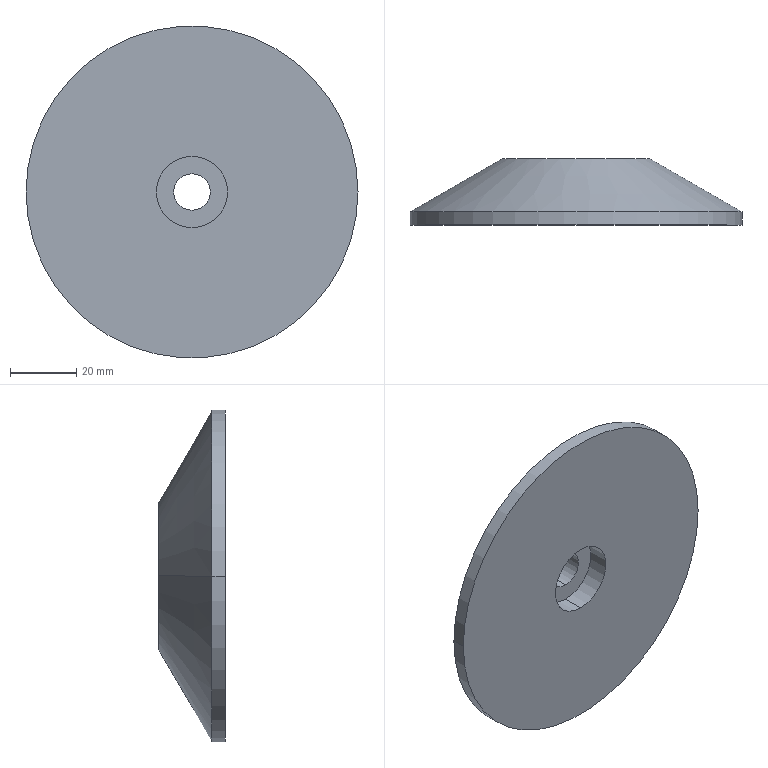Part | STEP file | Microwave Drying Flat Conveyor-CN2500x400-105-106 | 1 solid | 11 faces | box 100 x 20 x 100 mm | volume 96687 mm3 | cylinder 6 | plane 3 | cone 2 | commonest cylinder face diameters 11 x2 21.475 x2 100 x2
STEP:
#1=CARTESIAN_POINT('',(0.,6.4,10.738));
#2=VERTEX_POINT('',#1);
#3=CARTESIAN_POINT('',(0.,6.4,-10.738));
#4=VERTEX_POINT('',#3);
#5=CARTESIAN_POINT('',(0.,6.4,0.));
#6=DIRECTION('',(0.,-1.,0.));
#7=DIRECTION('',(0.,0.,-1.));
#8=AXIS2_PLACEMENT_3D('',#5,#6,#7);
#9=CIRCLE('',#8,10.738);
#10=EDGE_CURVE('',#2,#4,#9,.T.);
#11=ORIENTED_EDGE('',*,*,#10,.F.);
#12=CARTESIAN_POINT('',(0.,0.,10.737));
#13=VERTEX_POINT('',#12);
#14=CARTESIAN_POINT('',(0.,0.,10.738));
#15=DIRECTION('',(0.,-1.,0.));
#16=VECTOR('',#15,1000.);
#17=LINE('',#14,#16);
#18=EDGE_CURVE('',#2,#13,#17,.T.);
#19=ORIENTED_EDGE('',*,*,#18,.T.);
#20=CARTESIAN_POINT('',(0.,0.,-10.737));
#21=VERTEX_POINT('',#20);
#22=CARTESIAN_POINT('',(0.,0.,0.));
#23=DIRECTION('',(0.,-1.,0.));
#24=DIRECTION('',(0.,0.,-1.));
#25=AXIS2_PLACEMENT_3D('',#22,#23,#24);
#26=CIRCLE('',#25,10.737);
#27=EDGE_CURVE('',#13,#21,#26,.T.);
#28=ORIENTED_EDGE('',*,*,#27,.T.);
#29=CARTESIAN_POINT('',(0.,0.,-10.738));
#30=DIRECTION('',(0.,-1.,0.));
#31=VECTOR('',#30,1000.);
#32=LINE('',#29,#31);
#33=EDGE_CURVE('',#4,#21,#32,.T.);
#34=ORIENTED_EDGE('',*,*,#33,.F.);
#35=EDGE_LOOP('',(#11,#19,#28,#34));
#36=FACE_OUTER_BOUND('',#35,.T.);
#37=CARTESIAN_POINT('',(0.,0.,0.));
#38=DIRECTION('',(0.,-1.,0.));
#39=DIRECTION('',(0.,0.,-1.));
#40=AXIS2_PLACEMENT_3D('',#37,#38,#39);
#41=CYLINDRICAL_SURFACE('',#40,10.738);
#42=ADVANCED_FACE('',(#36),#41,.F.);
#43=CARTESIAN_POINT('',(0.,20.,5.5));
#44=VERTEX_POINT('',#43);
#45=CARTESIAN_POINT('',(0.,20.,-5.5));
#46=VERTEX_POINT('',#45);
#47=CARTESIAN_POINT('',(0.,20.,0.));
#48=DIRECTION('',(0.,-1.,0.));
#49=DIRECTION('',(0.,0.,-1.));
#50=AXIS2_PLACEMENT_3D('',#47,#48,#49);
#51=CIRCLE('',#50,5.5);
#52=EDGE_CURVE('',#44,#46,#51,.T.);
#53=ORIENTED_EDGE('',*,*,#52,.F.);
#54=CARTESIAN_POINT('',(0.,6.4,5.5));
#55=VERTEX_POINT('',#54);
#56=CARTESIAN_POINT('',(0.,0.,5.5));
#57=DIRECTION('',(0.,-1.,0.));
#58=VECTOR('',#57,1000.);
#59=LINE('',#56,#58);
#60=EDGE_CURVE('',#44,#55,#59,.T.);
#61=ORIENTED_EDGE('',*,*,#60,.T.);
#62=CARTESIAN_POINT('',(0.,6.4,-5.5));
#63=VERTEX_POINT('',#62);
#64=CARTESIAN_POINT('',(0.,6.4,0.));
#65=DIRECTION('',(0.,-1.,0.));
#66=DIRECTION('',(0.,0.,-1.));
#67=AXIS2_PLACEMENT_3D('',#64,#65,#66);
#68=CIRCLE('',#67,5.5);
#69=EDGE_CURVE('',#55,#63,#68,.T.);
#70=ORIENTED_EDGE('',*,*,#69,.T.);
#71=CARTESIAN_POINT('',(0.,0.,-5.5));
#72=DIRECTION('',(0.,-1.,0.));
#73=VECTOR('',#72,1000.);
#74=LINE('',#71,#73);
#75=EDGE_CURVE('',#46,#63,#74,.T.);
#76=ORIENTED_EDGE('',*,*,#75,.F.);
#77=EDGE_LOOP('',(#53,#61,#70,#76));
#78=FACE_OUTER_BOUND('',#77,.T.);
#79=CARTESIAN_POINT('',(0.,0.,0.));
#80=DIRECTION('',(0.,-1.,0.));
#81=DIRECTION('',(0.,0.,-1.));
#82=AXIS2_PLACEMENT_3D('',#79,#80,#81);
#83=CYLINDRICAL_SURFACE('',#82,5.5);
#84=ADVANCED_FACE('',(#78),#83,.F.);
#85=CARTESIAN_POINT('',(-22.287,20.,0.));
#86=VERTEX_POINT('',#85);
#87=CARTESIAN_POINT('',(22.287,20.,0.));
#88=VERTEX_POINT('',#87);
#89=CARTESIAN_POINT('',(0.,20.,0.));
#90=DIRECTION('',(0.,1.,0.));
#91=DIRECTION('',(-1.,0.,0.));
#92=AXIS2_PLACEMENT_3D('',#89,#90,#91);
#93=CIRCLE('',#92,22.287);
#94=EDGE_CURVE('',#86,#88,#93,.T.);
#95=ORIENTED_EDGE('',*,*,#94,.F.);
#96=CARTESIAN_POINT('',(-50.,4.,0.));
#97=VERTEX_POINT('',#96);
#98=CARTESIAN_POINT('',(-50.,4.,0.));
#99=DIRECTION('',(-0.866,-0.5,0.));
#100=VECTOR('',#99,1000.);
#101=LINE('',#98,#100);
#102=EDGE_CURVE('',#86,#97,#101,.T.);
#103=ORIENTED_EDGE('',*,*,#102,.T.);
#104=CARTESIAN_POINT('',(50.,4.,0.));
#105=VERTEX_POINT('',#104);
#106=CARTESIAN_POINT('',(0.,4.,0.));
#107=DIRECTION('',(0.,1.,0.));
#108=DIRECTION('',(-1.,0.,0.));
#109=AXIS2_PLACEMENT_3D('',#106,#107,#108);
#110=CIRCLE('',#109,50.);
#111=EDGE_CURVE('',#97,#105,#110,.T.);
#112=ORIENTED_EDGE('',*,*,#111,.T.);
#113=CARTESIAN_POINT('',(50.,4.,0.));
#114=DIRECTION('',(0.866,-0.5,0.));
#115=VECTOR('',#114,1000.);
#116=LINE('',#113,#115);
#117=EDGE_CURVE('',#88,#105,#116,.T.);
#118=ORIENTED_EDGE('',*,*,#117,.F.);
#119=EDGE_LOOP('',(#95,#103,#112,#118));
#120=FACE_OUTER_BOUND('',#119,.T.);
#121=CARTESIAN_POINT('',(0.,4.,0.));
#122=DIRECTION('',(0.,-1.,0.));
#123=DIRECTION('',(1.,0.,0.));
#124=AXIS2_PLACEMENT_3D('',#121,#122,#123);
#125=CONICAL_SURFACE('',#124,50.,1.047);
#126=ADVANCED_FACE('',(#120),#125,.T.);
#127=CARTESIAN_POINT('',(-50.,0.,0.));
#128=VERTEX_POINT('',#127);
#129=CARTESIAN_POINT('',(50.,0.,0.));
#130=VERTEX_POINT('',#129);
#131=CARTESIAN_POINT('',(0.,0.,0.));
#132=DIRECTION('',(0.,1.,0.));
#133=DIRECTION('',(-1.,0.,0.));
#134=AXIS2_PLACEMENT_3D('',#131,#132,#133);
#135=CIRCLE('',#134,50.);
#136=EDGE_CURVE('',#128,#130,#135,.T.);
#137=ORIENTED_EDGE('',*,*,#136,.T.);
#138=CARTESIAN_POINT('',(50.,20.,0.));
#139=DIRECTION('',(0.,1.,0.));
#140=VECTOR('',#139,1000.);
#141=LINE('',#138,#140);
#142=EDGE_CURVE('',#130,#105,#141,.T.);
#143=ORIENTED_EDGE('',*,*,#142,.T.);
#144=ORIENTED_EDGE('',*,*,#111,.F.);
#145=CARTESIAN_POINT('',(-50.,20.,0.));
#146=DIRECTION('',(0.,1.,0.));
#147=VECTOR('',#146,1000.);
#148=LINE('',#145,#147);
#149=EDGE_CURVE('',#128,#97,#148,.T.);
#150=ORIENTED_EDGE('',*,*,#149,.F.);
#151=EDGE_LOOP('',(#137,#143,#144,#150));
#152=FACE_OUTER_BOUND('',#151,.T.);
#153=CARTESIAN_POINT('',(0.,20.,0.));
#154=DIRECTION('',(0.,1.,0.));
#155=DIRECTION('',(-1.,0.,0.));
#156=AXIS2_PLACEMENT_3D('',#153,#154,#155);
#157=CYLINDRICAL_SURFACE('',#156,50.);
#158=ADVANCED_FACE('',(#152),#157,.T.);
#159=CARTESIAN_POINT('',(0.,0.,0.));
#160=DIRECTION('',(0.,-1.,0.));
#161=DIRECTION('',(0.,0.,-1.));
#162=AXIS2_PLACEMENT_3D('',#159,#160,#161);
#163=CIRCLE('',#162,10.737);
#164=EDGE_CURVE('',#21,#13,#163,.T.);
#165=ORIENTED_EDGE('',*,*,#164,.F.);
#166=ORIENTED_EDGE('',*,*,#27,.F.);
#167=EDGE_LOOP('',(#165,#166));
#168=FACE_BOUND('',#167,.T.);
#169=ORIENTED_EDGE('',*,*,#136,.F.);
#170=CARTESIAN_POINT('',(0.,0.,0.));
#171=DIRECTION('',(0.,1.,0.));
#172=DIRECTION('',(-1.,0.,0.));
#173=AXIS2_PLACEMENT_3D('',#170,#171,#172);
#174=CIRCLE('',#173,50.);
#175=EDGE_CURVE('',#130,#128,#174,.T.);
#176=ORIENTED_EDGE('',*,*,#175,.F.);
#177=EDGE_LOOP('',(#169,#176));
#178=FACE_OUTER_BOUND('',#177,.T.);
#179=CARTESIAN_POINT('',(0.,0.,0.));
#180=DIRECTION('',(0.,1.,0.));
#181=DIRECTION('',(-1.,0.,0.));
#182=AXIS2_PLACEMENT_3D('',#179,#180,#181);
#183=PLANE('',#182);
#184=ADVANCED_FACE('',(#168,#178),#183,.F.);
#185=ORIENTED_EDGE('',*,*,#142,.F.);
#186=ORIENTED_EDGE('',*,*,#175,.T.);
#187=ORIENTED_EDGE('',*,*,#149,.T.);
#188=CARTESIAN_POINT('',(0.,4.,0.));
#189=DIRECTION('',(0.,1.,0.));
#190=DIRECTION('',(-1.,0.,0.));
#191=AXIS2_PLACEMENT_3D('',#188,#189,#190);
#192=CIRCLE('',#191,50.);
#193=EDGE_CURVE('',#105,#97,#192,.T.);
#194=ORIENTED_EDGE('',*,*,#193,.F.);
#195=EDGE_LOOP('',(#185,#186,#187,#194));
#196=FACE_OUTER_BOUND('',#195,.T.);
#197=CARTESIAN_POINT('',(0.,20.,0.));
#198=DIRECTION('',(0.,1.,0.));
#199=DIRECTION('',(-1.,0.,0.));
#200=AXIS2_PLACEMENT_3D('',#197,#198,#199);
#201=CYLINDRICAL_SURFACE('',#200,50.);
#202=ADVANCED_FACE('',(#196),#201,.T.);
#203=ORIENTED_EDGE('',*,*,#102,.F.);
#204=CARTESIAN_POINT('',(0.,20.,0.));
#205=DIRECTION('',(0.,1.,0.));
#206=DIRECTION('',(-1.,0.,0.));
#207=AXIS2_PLACEMENT_3D('',#204,#205,#206);
#208=CIRCLE('',#207,22.287);
#209=EDGE_CURVE('',#88,#86,#208,.T.);
#210=ORIENTED_EDGE('',*,*,#209,.F.);
#211=ORIENTED_EDGE('',*,*,#117,.T.);
#212=ORIENTED_EDGE('',*,*,#193,.T.);
#213=EDGE_LOOP('',(#203,#210,#211,#212));
#214=FACE_OUTER_BOUND('',#213,.T.);
#215=CARTESIAN_POINT('',(0.,4.,0.));
#216=DIRECTION('',(0.,-1.,0.));
#217=DIRECTION('',(1.,0.,0.));
#218=AXIS2_PLACEMENT_3D('',#215,#216,#217);
#219=CONICAL_SURFACE('',#218,50.,1.047);
#220=ADVANCED_FACE('',(#214),#219,.T.);
#221=CARTESIAN_POINT('',(0.,20.,0.));
#222=DIRECTION('',(0.,-1.,0.));
#223=DIRECTION('',(0.,0.,-1.));
#224=AXIS2_PLACEMENT_3D('',#221,#222,#223);
#225=CIRCLE('',#224,5.5);
#226=EDGE_CURVE('',#46,#44,#225,.T.);
#227=ORIENTED_EDGE('',*,*,#226,.T.);
#228=ORIENTED_EDGE('',*,*,#52,.T.);
#229=EDGE_LOOP('',(#227,#228));
#230=FACE_BOUND('',#229,.T.);
#231=ORIENTED_EDGE('',*,*,#209,.T.);
#232=ORIENTED_EDGE('',*,*,#94,.T.);
#233=EDGE_LOOP('',(#231,#232));
#234=FACE_OUTER_BOUND('',#233,.T.);
#235=CARTESIAN_POINT('',(22.287,20.,0.));
#236=DIRECTION('',(0.,-1.,0.));
#237=DIRECTION('',(1.,0.,0.));
#238=AXIS2_PLACEMENT_3D('',#235,#236,#237);
#239=PLANE('',#238);
#240=ADVANCED_FACE('',(#230,#234),#239,.F.);
#241=ORIENTED_EDGE('',*,*,#60,.F.);
#242=ORIENTED_EDGE('',*,*,#226,.F.);
#243=ORIENTED_EDGE('',*,*,#75,.T.);
#244=CARTESIAN_POINT('',(0.,6.4,0.));
#245=DIRECTION('',(0.,-1.,0.));
#246=DIRECTION('',(0.,0.,-1.));
#247=AXIS2_PLACEMENT_3D('',#244,#245,#246);
#248=CIRCLE('',#247,5.5);
#249=EDGE_CURVE('',#63,#55,#248,.T.);
#250=ORIENTED_EDGE('',*,*,#249,.T.);
#251=EDGE_LOOP('',(#241,#242,#243,#250));
#252=FACE_OUTER_BOUND('',#251,.T.);
#253=CARTESIAN_POINT('',(0.,0.,0.));
#254=DIRECTION('',(0.,-1.,0.));
#255=DIRECTION('',(0.,0.,-1.));
#256=AXIS2_PLACEMENT_3D('',#253,#254,#255);
#257=CYLINDRICAL_SURFACE('',#256,5.5);
#258=ADVANCED_FACE('',(#252),#257,.F.);
#259=ORIENTED_EDGE('',*,*,#249,.F.);
#260=ORIENTED_EDGE('',*,*,#69,.F.);
#261=EDGE_LOOP('',(#259,#260));
#262=FACE_BOUND('',#261,.T.);
#263=CARTESIAN_POINT('',(0.,6.4,0.));
#264=DIRECTION('',(0.,-1.,0.));
#265=DIRECTION('',(0.,0.,-1.));
#266=AXIS2_PLACEMENT_3D('',#263,#264,#265);
#267=CIRCLE('',#266,10.738);
#268=EDGE_CURVE('',#4,#2,#267,.T.);
#269=ORIENTED_EDGE('',*,*,#268,.T.);
#270=ORIENTED_EDGE('',*,*,#10,.T.);
#271=EDGE_LOOP('',(#269,#270));
#272=FACE_OUTER_BOUND('',#271,.T.);
#273=CARTESIAN_POINT('',(5.5,6.4,0.));
#274=DIRECTION('',(0.,1.,0.));
#275=DIRECTION('',(0.,0.,1.));
#276=AXIS2_PLACEMENT_3D('',#273,#274,#275);
#277=PLANE('',#276);
#278=ADVANCED_FACE('',(#262,#272),#277,.F.);
#279=ORIENTED_EDGE('',*,*,#18,.F.);
#280=ORIENTED_EDGE('',*,*,#268,.F.);
#281=ORIENTED_EDGE('',*,*,#33,.T.);
#282=ORIENTED_EDGE('',*,*,#164,.T.);
#283=EDGE_LOOP('',(#279,#280,#281,#282));
#284=FACE_OUTER_BOUND('',#283,.T.);
#285=CARTESIAN_POINT('',(0.,0.,0.));
#286=DIRECTION('',(0.,-1.,0.));
#287=DIRECTION('',(0.,0.,-1.));
#288=AXIS2_PLACEMENT_3D('',#285,#286,#287);
#289=CYLINDRICAL_SURFACE('',#288,10.738);
#290=ADVANCED_FACE('',(#284),#289,.F.);
#291=CLOSED_SHELL('',(#42,#84,#126,#158,#184,#202,#220,#240,#258,#278,#290));
#292=MANIFOLD_SOLID_BREP('',#291);
#293=CARTESIAN_POINT('',(0.,0.,0.));
#294=DIRECTION('',(0.,0.,1.));
#295=DIRECTION('',(1.,0.,0.));
#296=AXIS2_PLACEMENT_3D('',#293,#294,#295);
#297=(LENGTH_UNIT()NAMED_UNIT(*)SI_UNIT(.MILLI.,.METRE.));
#298=UNCERTAINTY_MEASURE_WITH_UNIT(LENGTH_MEASURE(0.00001),#297,'','');
#299=(NAMED_UNIT(*)PLANE_ANGLE_UNIT()SI_UNIT($,.RADIAN.));
#300=(NAMED_UNIT(*)SI_UNIT($,.STERADIAN.)SOLID_ANGLE_UNIT());
#301=(GEOMETRIC_REPRESENTATION_CONTEXT(3)GLOBAL_UNCERTAINTY_ASSIGNED_CONTEXT((#298))GLOBAL_UNIT_ASSIGNED_CONTEXT((#297,#299,#300))REPRESENTATION_CONTEXT('',''));
#302=ADVANCED_BREP_SHAPE_REPRESENTATION('',(#292,#296),#301);